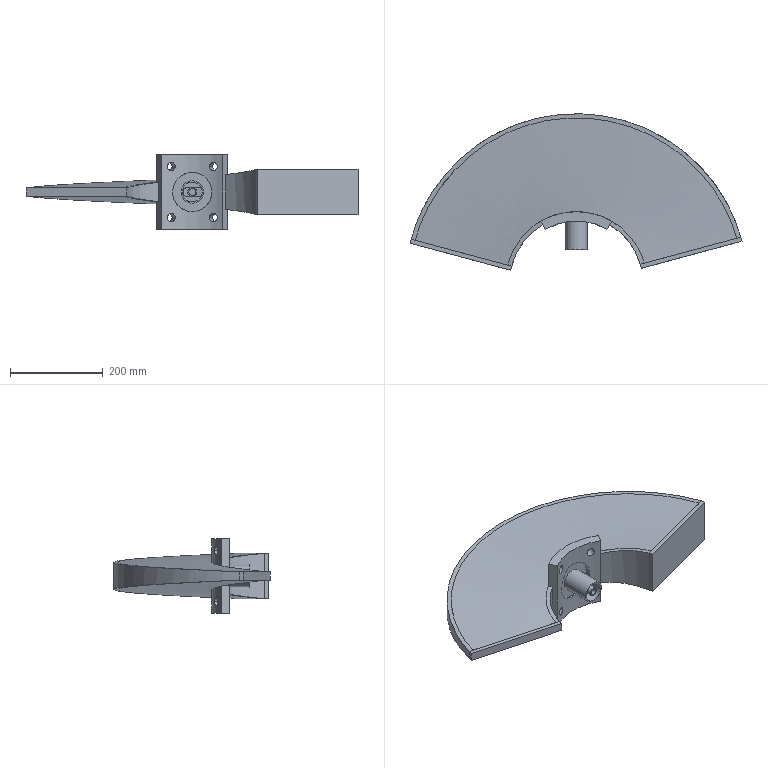Part | SolidWorks | features ICE 17, MoveFace 13, DeleteBody 4, Chamfer 2, OffsetRefSurface 2, Split 2, Thicken 2, Blend 1, CirPattern 1, CombineBodies 1, Extrusion 1, MirrorSolid 1, Punch 1, RefAxis 1, RevCut 1, WeldmentFeature 1 | 8 solids | 75 faces | box 715.716 x 337.387 x 160 mm | volume 3757176 mm3 | plane 30 | cylinder 27 | spline 18 | commonest cylinder face diameters 18 x8 20 x3 15 x2 19 x2 43 x2 48 x2